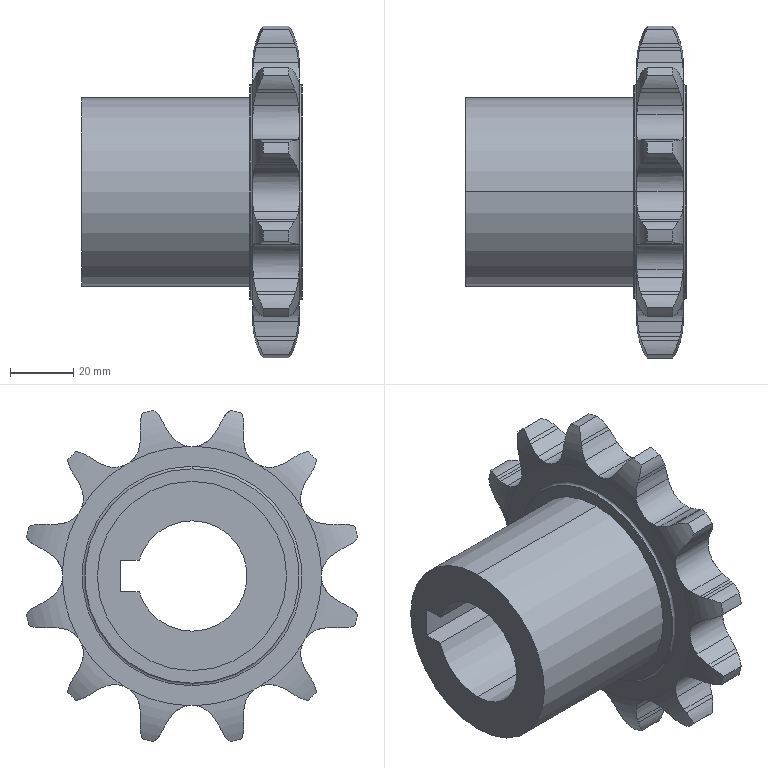Part | STEP file | Drive sprocket 16A-12_05B | 1 solid | 148 faces | box 70 x 105.245 x 105.245 mm | volume 183354 mm3 | cylinder 88 | plane 32 | torus 28 | commonest cylinder face diameters 23.691 x26 41.467 x26 16.059 x15 108 x12 68 x4 35 x3